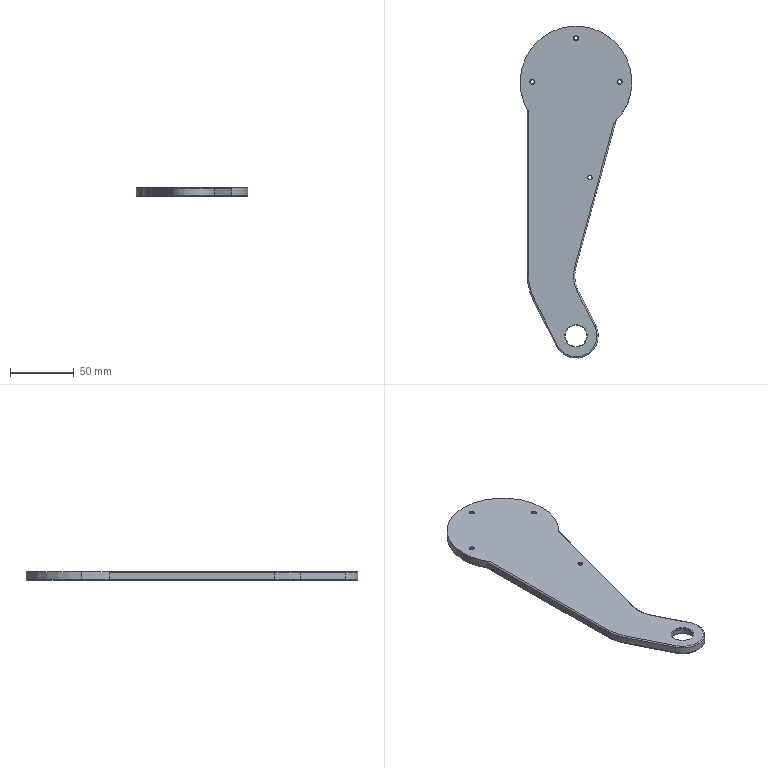Part | SolidWorks | features Fillet 5, ICE 3, Extrusion 1 | 1 solid | 96 faces | box 88 x 261.5 x 7 mm | volume 97457 mm3 | torus 51 | cylinder 34 | plane 11 | commonest cylinder face diameters 2 x8 7 x8 3.2 x6 88 x3 3.1 x2 17 x2